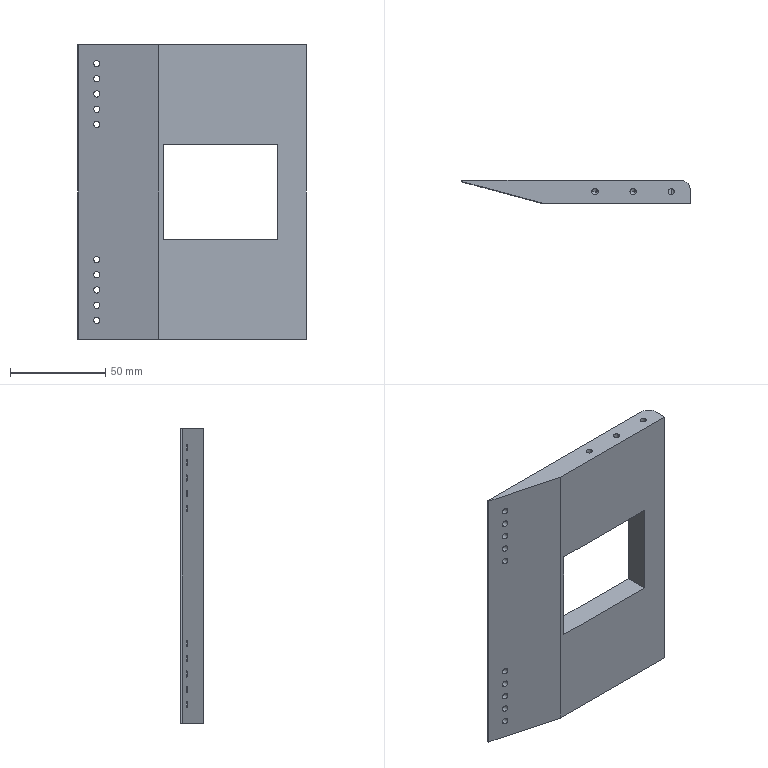Part | STEP file | MT-COMBO-119-S038 | 1 solid | 99 faces | box 120 x 12 x 155 mm | volume 147093 mm3 | cylinder 60 | cone 28 | plane 11 | commonest cylinder face diameters 3.3 x58 1.5 x1 10 x1